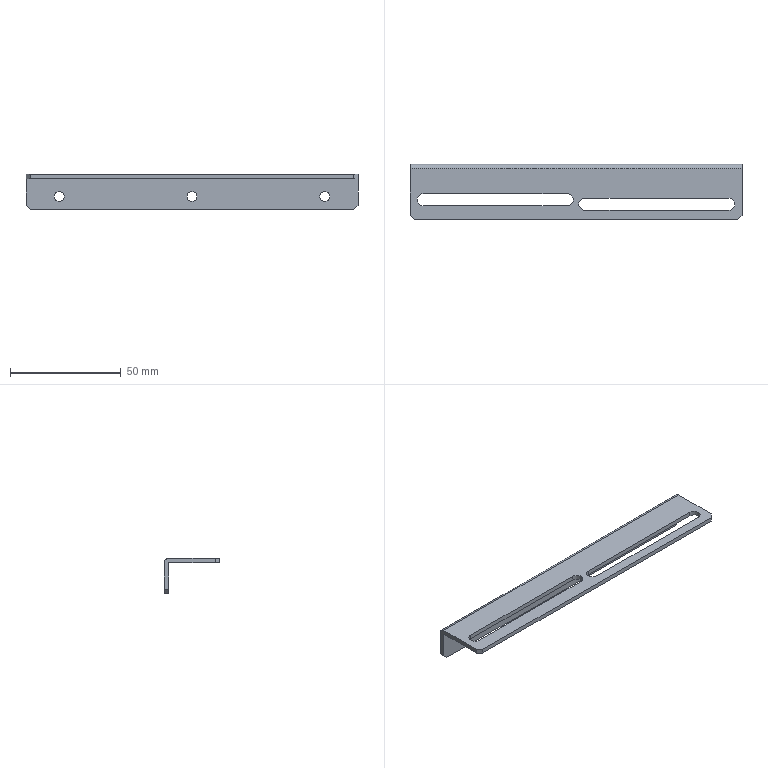Part | SolidWorks | features ICE 4, Chamfer 3, HoleWzd 3, Extrusion 1, Fillet 1 | 1 solid | 29 faces | box 150 x 25 x 16 mm | volume 9935 mm3 | plane 16 | cylinder 13 | commonest cylinder face diameters 4.5 x6 5.5 x6 4 x1
STEP:
#1=CARTESIAN_POINT('',(0.,10.5,5.75));
#2=VERTEX_POINT('',#1);
#3=CARTESIAN_POINT('',(0.,10.5,10.25));
#4=VERTEX_POINT('',#3);
#5=CARTESIAN_POINT('',(0.,10.5,8.));
#6=DIRECTION('',(0.,1.,0.));
#7=DIRECTION('',(0.,0.,1.));
#8=AXIS2_PLACEMENT_3D('',#5,#6,#7);
#9=CIRCLE('',#8,2.25);
#10=EDGE_CURVE('',#2,#4,#9,.T.);
#11=ORIENTED_EDGE('',*,*,#10,.F.);
#12=CARTESIAN_POINT('',(0.,12.5,5.75));
#13=VERTEX_POINT('',#12);
#14=CARTESIAN_POINT('',(0.,12.5,5.75));
#15=DIRECTION('',(0.,1.,0.));
#16=VECTOR('',#15,1000.);
#17=LINE('',#14,#16);
#18=EDGE_CURVE('',#2,#13,#17,.T.);
#19=ORIENTED_EDGE('',*,*,#18,.T.);
#20=CARTESIAN_POINT('',(0.,12.5,10.25));
#21=VERTEX_POINT('',#20);
#22=CARTESIAN_POINT('',(0.,12.5,8.));
#23=DIRECTION('',(0.,1.,0.));
#24=DIRECTION('',(0.,0.,1.));
#25=AXIS2_PLACEMENT_3D('',#22,#23,#24);
#26=CIRCLE('',#25,2.25);
#27=EDGE_CURVE('',#13,#21,#26,.T.);
#28=ORIENTED_EDGE('',*,*,#27,.T.);
#29=CARTESIAN_POINT('',(0.,12.5,10.25));
#30=DIRECTION('',(0.,1.,0.));
#31=VECTOR('',#30,1000.);
#32=LINE('',#29,#31);
#33=EDGE_CURVE('',#4,#21,#32,.T.);
#34=ORIENTED_EDGE('',*,*,#33,.F.);
#35=EDGE_LOOP('',(#11,#19,#28,#34));
#36=FACE_OUTER_BOUND('',#35,.T.);
#37=CARTESIAN_POINT('',(0.,12.5,8.));
#38=DIRECTION('',(0.,1.,0.));
#39=DIRECTION('',(0.,0.,1.));
#40=AXIS2_PLACEMENT_3D('',#37,#38,#39);
#41=CYLINDRICAL_SURFACE('',#40,2.25);
#42=ADVANCED_FACE('',(#36),#41,.F.);
#43=CARTESIAN_POINT('',(-60.,10.5,5.75));
#44=VERTEX_POINT('',#43);
#45=CARTESIAN_POINT('',(-60.,10.5,10.25));
#46=VERTEX_POINT('',#45);
#47=CARTESIAN_POINT('',(-60.,10.5,8.));
#48=DIRECTION('',(0.,1.,0.));
#49=DIRECTION('',(0.,0.,1.));
#50=AXIS2_PLACEMENT_3D('',#47,#48,#49);
#51=CIRCLE('',#50,2.25);
#52=EDGE_CURVE('',#44,#46,#51,.T.);
#53=ORIENTED_EDGE('',*,*,#52,.F.);
#54=CARTESIAN_POINT('',(-60.,12.5,5.75));
#55=VERTEX_POINT('',#54);
#56=CARTESIAN_POINT('',(-60.,12.5,5.75));
#57=DIRECTION('',(0.,1.,0.));
#58=VECTOR('',#57,1000.);
#59=LINE('',#56,#58);
#60=EDGE_CURVE('',#44,#55,#59,.T.);
#61=ORIENTED_EDGE('',*,*,#60,.T.);
#62=CARTESIAN_POINT('',(-60.,12.5,10.25));
#63=VERTEX_POINT('',#62);
#64=CARTESIAN_POINT('',(-60.,12.5,8.));
#65=DIRECTION('',(0.,1.,0.));
#66=DIRECTION('',(0.,0.,1.));
#67=AXIS2_PLACEMENT_3D('',#64,#65,#66);
#68=CIRCLE('',#67,2.25);
#69=EDGE_CURVE('',#55,#63,#68,.T.);
#70=ORIENTED_EDGE('',*,*,#69,.T.);
#71=CARTESIAN_POINT('',(-60.,12.5,10.25));
#72=DIRECTION('',(0.,1.,0.));
#73=VECTOR('',#72,1000.);
#74=LINE('',#71,#73);
#75=EDGE_CURVE('',#46,#63,#74,.T.);
#76=ORIENTED_EDGE('',*,*,#75,.F.);
#77=EDGE_LOOP('',(#53,#61,#70,#76));
#78=FACE_OUTER_BOUND('',#77,.T.);
#79=CARTESIAN_POINT('',(-60.,12.5,8.));
#80=DIRECTION('',(0.,1.,0.));
#81=DIRECTION('',(0.,0.,1.));
#82=AXIS2_PLACEMENT_3D('',#79,#80,#81);
#83=CYLINDRICAL_SURFACE('',#82,2.25);
#84=ADVANCED_FACE('',(#78),#83,.F.);
#85=CARTESIAN_POINT('',(60.,10.5,5.75));
#86=VERTEX_POINT('',#85);
#87=CARTESIAN_POINT('',(60.,10.5,10.25));
#88=VERTEX_POINT('',#87);
#89=CARTESIAN_POINT('',(60.,10.5,8.));
#90=DIRECTION('',(0.,1.,0.));
#91=DIRECTION('',(0.,0.,1.));
#92=AXIS2_PLACEMENT_3D('',#89,#90,#91);
#93=CIRCLE('',#92,2.25);
#94=EDGE_CURVE('',#86,#88,#93,.T.);
#95=ORIENTED_EDGE('',*,*,#94,.F.);
#96=CARTESIAN_POINT('',(60.,12.5,5.75));
#97=VERTEX_POINT('',#96);
#98=CARTESIAN_POINT('',(60.,12.5,5.75));
#99=DIRECTION('',(0.,1.,0.));
#100=VECTOR('',#99,1000.);
#101=LINE('',#98,#100);
#102=EDGE_CURVE('',#86,#97,#101,.T.);
#103=ORIENTED_EDGE('',*,*,#102,.T.);
#104=CARTESIAN_POINT('',(60.,12.5,10.25));
#105=VERTEX_POINT('',#104);
#106=CARTESIAN_POINT('',(60.,12.5,8.));
#107=DIRECTION('',(0.,1.,0.));
#108=DIRECTION('',(0.,0.,1.));
#109=AXIS2_PLACEMENT_3D('',#106,#107,#108);
#110=CIRCLE('',#109,2.25);
#111=EDGE_CURVE('',#97,#105,#110,.T.);
#112=ORIENTED_EDGE('',*,*,#111,.T.);
#113=CARTESIAN_POINT('',(60.,12.5,10.25));
#114=DIRECTION('',(0.,1.,0.));
#115=VECTOR('',#114,1000.);
#116=LINE('',#113,#115);
#117=EDGE_CURVE('',#88,#105,#116,.T.);
#118=ORIENTED_EDGE('',*,*,#117,.F.);
#119=EDGE_LOOP('',(#95,#103,#112,#118));
#120=FACE_OUTER_BOUND('',#119,.T.);
#121=CARTESIAN_POINT('',(60.,12.5,8.));
#122=DIRECTION('',(0.,1.,0.));
#123=DIRECTION('',(0.,0.,1.));
#124=AXIS2_PLACEMENT_3D('',#121,#122,#123);
#125=CYLINDRICAL_SURFACE('',#124,2.25);
#126=ADVANCED_FACE('',(#120),#125,.F.);
#127=CARTESIAN_POINT('',(-1.25,-3.5,16.));
#128=VERTEX_POINT('',#127);
#129=CARTESIAN_POINT('',(-4.,-0.75,16.));
#130=VERTEX_POINT('',#129);
#131=CARTESIAN_POINT('',(-4.,-3.5,16.));
#132=DIRECTION('',(0.,0.,1.));
#133=DIRECTION('',(1.,0.,0.));
#134=AXIS2_PLACEMENT_3D('',#131,#132,#133);
#135=CIRCLE('',#134,2.75);
#136=EDGE_CURVE('',#128,#130,#135,.T.);
#137=ORIENTED_EDGE('',*,*,#136,.F.);
#138=CARTESIAN_POINT('',(-1.25,-3.5,18.));
#139=VERTEX_POINT('',#138);
#140=CARTESIAN_POINT('',(-1.25,-3.5,0.));
#141=DIRECTION('',(0.,0.,1.));
#142=VECTOR('',#141,1000.);
#143=LINE('',#140,#142);
#144=EDGE_CURVE('',#128,#139,#143,.T.);
#145=ORIENTED_EDGE('',*,*,#144,.T.);
#146=CARTESIAN_POINT('',(-4.,-0.75,18.));
#147=VERTEX_POINT('',#146);
#148=CARTESIAN_POINT('',(-4.,-3.5,18.));
#149=DIRECTION('',(0.,0.,1.));
#150=DIRECTION('',(1.,0.,0.));
#151=AXIS2_PLACEMENT_3D('',#148,#149,#150);
#152=CIRCLE('',#151,2.75);
#153=EDGE_CURVE('',#139,#147,#152,.T.);
#154=ORIENTED_EDGE('',*,*,#153,.T.);
#155=CARTESIAN_POINT('',(-4.,-0.75,0.));
#156=DIRECTION('',(0.,0.,1.));
#157=VECTOR('',#156,1000.);
#158=LINE('',#155,#157);
#159=EDGE_CURVE('',#130,#147,#158,.T.);
#160=ORIENTED_EDGE('',*,*,#159,.F.);
#161=EDGE_LOOP('',(#137,#145,#154,#160));
#162=FACE_OUTER_BOUND('',#161,.T.);
#163=CARTESIAN_POINT('',(-4.,-3.5,0.));
#164=DIRECTION('',(0.,0.,1.));
#165=DIRECTION('',(1.,0.,0.));
#166=AXIS2_PLACEMENT_3D('',#163,#164,#165);
#167=CYLINDRICAL_SURFACE('',#166,2.75);
#168=ADVANCED_FACE('',(#162),#167,.F.);
#169=CARTESIAN_POINT('',(1.25,-5.5,18.));
#170=VERTEX_POINT('',#169);
#171=CARTESIAN_POINT('',(4.,-2.75,18.));
#172=VERTEX_POINT('',#171);
#173=CARTESIAN_POINT('',(4.,-5.5,18.));
#174=DIRECTION('',(0.,0.,-1.));
#175=DIRECTION('',(-1.,0.,0.));
#176=AXIS2_PLACEMENT_3D('',#173,#174,#175);
#177=CIRCLE('',#176,2.75);
#178=EDGE_CURVE('',#170,#172,#177,.T.);
#179=ORIENTED_EDGE('',*,*,#178,.F.);
#180=CARTESIAN_POINT('',(1.25,-5.5,16.));
#181=VERTEX_POINT('',#180);
#182=CARTESIAN_POINT('',(1.25,-5.5,18.));
#183=DIRECTION('',(0.,0.,-1.));
#184=VECTOR('',#183,1000.);
#185=LINE('',#182,#184);
#186=EDGE_CURVE('',#170,#181,#185,.T.);
#187=ORIENTED_EDGE('',*,*,#186,.T.);
#188=CARTESIAN_POINT('',(4.,-2.75,16.));
#189=VERTEX_POINT('',#188);
#190=CARTESIAN_POINT('',(4.,-5.5,16.));
#191=DIRECTION('',(0.,0.,-1.));
#192=DIRECTION('',(-1.,0.,0.));
#193=AXIS2_PLACEMENT_3D('',#190,#191,#192);
#194=CIRCLE('',#193,2.75);
#195=EDGE_CURVE('',#181,#189,#194,.T.);
#196=ORIENTED_EDGE('',*,*,#195,.T.);
#197=CARTESIAN_POINT('',(4.,-2.75,18.));
#198=DIRECTION('',(0.,0.,-1.));
#199=VECTOR('',#198,1000.);
#200=LINE('',#197,#199);
#201=EDGE_CURVE('',#172,#189,#200,.T.);
#202=ORIENTED_EDGE('',*,*,#201,.F.);
#203=EDGE_LOOP('',(#179,#187,#196,#202));
#204=FACE_OUTER_BOUND('',#203,.T.);
#205=CARTESIAN_POINT('',(4.,-5.5,18.));
#206=DIRECTION('',(0.,0.,-1.));
#207=DIRECTION('',(-1.,0.,0.));
#208=AXIS2_PLACEMENT_3D('',#205,#206,#207);
#209=CYLINDRICAL_SURFACE('',#208,2.75);
#210=ADVANCED_FACE('',(#204),#209,.F.);
#211=CARTESIAN_POINT('',(-75.,12.5,16.));
#212=VERTEX_POINT('',#211);
#213=CARTESIAN_POINT('',(-75.,12.5,4.));
#214=VERTEX_POINT('',#213);
#215=CARTESIAN_POINT('',(-75.,12.5,18.));
#216=DIRECTION('',(0.,0.,-1.));
#217=VECTOR('',#216,1000.);
#218=LINE('',#215,#217);
#219=EDGE_CURVE('',#212,#214,#218,.T.);
#220=ORIENTED_EDGE('',*,*,#219,.T.);
#221=CARTESIAN_POINT('',(-75.,10.5,4.));
#222=VERTEX_POINT('',#221);
#223=CARTESIAN_POINT('',(-75.,10.5,4.));
#224=DIRECTION('',(0.,-1.,0.));
#225=VECTOR('',#224,1000.);
#226=LINE('',#223,#225);
#227=EDGE_CURVE('',#214,#222,#226,.T.);
#228=ORIENTED_EDGE('',*,*,#227,.T.);
#229=CARTESIAN_POINT('',(-75.,10.5,16.));
#230=VERTEX_POINT('',#229);
#231=CARTESIAN_POINT('',(-75.,10.5,16.));
#232=DIRECTION('',(0.,0.,-1.));
#233=VECTOR('',#232,1000.);
#234=LINE('',#231,#233);
#235=EDGE_CURVE('',#230,#222,#234,.T.);
#236=ORIENTED_EDGE('',*,*,#235,.F.);
#237=CARTESIAN_POINT('',(-75.,-10.5,16.));
#238=VERTEX_POINT('',#237);
#239=CARTESIAN_POINT('',(-75.,-12.5,16.));
#240=DIRECTION('',(0.,1.,0.));
#241=VECTOR('',#240,1000.);
#242=LINE('',#239,#241);
#243=EDGE_CURVE('',#238,#230,#242,.T.);
#244=ORIENTED_EDGE('',*,*,#243,.F.);
#245=CARTESIAN_POINT('',(-75.,-10.5,18.));
#246=VERTEX_POINT('',#245);
#247=CARTESIAN_POINT('',(-75.,-10.5,18.));
#248=DIRECTION('',(0.,0.,1.));
#249=VECTOR('',#248,1000.);
#250=LINE('',#247,#249);
#251=EDGE_CURVE('',#238,#246,#250,.T.);
#252=ORIENTED_EDGE('',*,*,#251,.T.);
#253=CARTESIAN_POINT('',(-75.,10.5,18.));
#254=VERTEX_POINT('',#253);
#255=CARTESIAN_POINT('',(-75.,-12.5,18.));
#256=DIRECTION('',(0.,1.,0.));
#257=VECTOR('',#256,1000.);
#258=LINE('',#255,#257);
#259=EDGE_CURVE('',#246,#254,#258,.T.);
#260=ORIENTED_EDGE('',*,*,#259,.T.);
#261=CARTESIAN_POINT('',(-75.,10.5,16.));
#262=DIRECTION('',(-1.,0.,0.));
#263=DIRECTION('',(0.,0.,1.));
#264=AXIS2_PLACEMENT_3D('',#261,#262,#263);
#265=CIRCLE('',#264,2.);
#266=EDGE_CURVE('',#254,#212,#265,.T.);
#267=ORIENTED_EDGE('',*,*,#266,.T.);
#268=EDGE_LOOP('',(#220,#228,#236,#244,#252,#260,#267));
#269=FACE_OUTER_BOUND('',#268,.T.);
#270=CARTESIAN_POINT('',(-75.,-12.5,18.));
#271=DIRECTION('',(-1.,0.,0.));
#272=DIRECTION('',(0.,0.,1.));
#273=AXIS2_PLACEMENT_3D('',#270,#271,#272);
#274=PLANE('',#273);
#275=ADVANCED_FACE('',(#269),#274,.T.);
#276=CARTESIAN_POINT('',(73.,-12.5,18.));
#277=VERTEX_POINT('',#276);
#278=CARTESIAN_POINT('',(-73.,-12.5,18.));
#279=VERTEX_POINT('',#278);
#280=CARTESIAN_POINT('',(75.,-12.5,18.));
#281=DIRECTION('',(-1.,0.,0.));
#282=VECTOR('',#281,1000.);
#283=LINE('',#280,#282);
#284=EDGE_CURVE('',#277,#279,#283,.T.);
#285=ORIENTED_EDGE('',*,*,#284,.T.);
#286=CARTESIAN_POINT('',(-73.,-12.5,16.));
#287=VERTEX_POINT('',#286);
#288=CARTESIAN_POINT('',(-73.,-12.5,18.));
#289=DIRECTION('',(0.,0.,-1.));
#290=VECTOR('',#289,1000.);
#291=LINE('',#288,#290);
#292=EDGE_CURVE('',#279,#287,#291,.T.);
#293=ORIENTED_EDGE('',*,*,#292,.T.);
#294=CARTESIAN_POINT('',(73.,-12.5,16.));
#295=VERTEX_POINT('',#294);
#296=CARTESIAN_POINT('',(75.,-12.5,16.));
#297=DIRECTION('',(-1.,0.,0.));
#298=VECTOR('',#297,1000.);
#299=LINE('',#296,#298);
#300=EDGE_CURVE('',#295,#287,#299,.T.);
#301=ORIENTED_EDGE('',*,*,#300,.F.);
#302=CARTESIAN_POINT('',(73.,-12.5,18.));
#303=DIRECTION('',(0.,0.,1.));
#304=VECTOR('',#303,1000.);
#305=LINE('',#302,#304);
#306=EDGE_CURVE('',#295,#277,#305,.T.);
#307=ORIENTED_EDGE('',*,*,#306,.T.);
#308=EDGE_LOOP('',(#285,#293,#301,#307));
#309=FACE_OUTER_BOUND('',#308,.T.);
#310=CARTESIAN_POINT('',(75.,-12.5,18.));
#311=DIRECTION('',(0.,-1.,0.));
#312=DIRECTION('',(0.,0.,-1.));
#313=AXIS2_PLACEMENT_3D('',#310,#311,#312);
#314=PLANE('',#313);
#315=ADVANCED_FACE('',(#309),#314,.T.);
#316=CARTESIAN_POINT('',(75.,10.5,16.));
#317=VERTEX_POINT('',#316);
#318=CARTESIAN_POINT('',(75.,10.5,4.));
#319=VERTEX_POINT('',#318);
#320=CARTESIAN_POINT('',(75.,10.5,16.));
#321=DIRECTION('',(0.,0.,-1.));
#322=VECTOR('',#321,1000.);
#323=LINE('',#320,#322);
#324=EDGE_CURVE('',#317,#319,#323,.T.);
#325=ORIENTED_EDGE('',*,*,#324,.T.);
#326=CARTESIAN_POINT('',(75.,12.5,4.));
#327=VERTEX_POINT('',#326);
#328=CARTESIAN_POINT('',(75.,12.5,4.));
#329=DIRECTION('',(0.,1.,0.));
#330=VECTOR('',#329,1000.);
#331=LINE('',#328,#330);
#332=EDGE_CURVE('',#319,#327,#331,.T.);
#333=ORIENTED_EDGE('',*,*,#332,.T.);
#334=CARTESIAN_POINT('',(75.,12.5,16.));
#335=VERTEX_POINT('',#334);
#336=CARTESIAN_POINT('',(75.,12.5,18.));
#337=DIRECTION('',(0.,0.,-1.));
#338=VECTOR('',#337,1000.);
#339=LINE('',#336,#338);
#340=EDGE_CURVE('',#335,#327,#339,.T.);
#341=ORIENTED_EDGE('',*,*,#340,.F.);
#342=CARTESIAN_POINT('',(75.,10.5,18.));
#343=VERTEX_POINT('',#342);
#344=CARTESIAN_POINT('',(75.,10.5,16.));
#345=DIRECTION('',(1.,0.,0.));
#346=DIRECTION('',(0.,0.,-1.));
#347=AXIS2_PLACEMENT_3D('',#344,#345,#346);
#348=CIRCLE('',#347,2.);
#349=EDGE_CURVE('',#335,#343,#348,.T.);
#350=ORIENTED_EDGE('',*,*,#349,.T.);
#351=CARTESIAN_POINT('',(75.,-10.5,18.));
#352=VERTEX_POINT('',#351);
#353=CARTESIAN_POINT('',(75.,12.5,18.));
#354=DIRECTION('',(0.,-1.,0.));
#355=VECTOR('',#354,1000.);
#356=LINE('',#353,#355);
#357=EDGE_CURVE('',#343,#352,#356,.T.);
#358=ORIENTED_EDGE('',*,*,#357,.T.);
#359=CARTESIAN_POINT('',(75.,-10.5,16.));
#360=VERTEX_POINT('',#359);
#361=CARTESIAN_POINT('',(75.,-10.5,18.));
#362=DIRECTION('',(0.,0.,-1.));
#363=VECTOR('',#362,1000.);
#364=LINE('',#361,#363);
#365=EDGE_CURVE('',#352,#360,#364,.T.);
#366=ORIENTED_EDGE('',*,*,#365,.T.);
#367=CARTESIAN_POINT('',(75.,-12.5,16.));
#368=DIRECTION('',(0.,1.,0.));
#369=VECTOR('',#368,1000.);
#370=LINE('',#367,#369);
#371=EDGE_CURVE('',#360,#317,#370,.T.);
#372=ORIENTED_EDGE('',*,*,#371,.T.);
#373=EDGE_LOOP('',(#325,#333,#341,#350,#358,#366,#372));
#374=FACE_OUTER_BOUND('',#373,.T.);
#375=CARTESIAN_POINT('',(75.,12.5,18.));
#376=DIRECTION('',(1.,0.,0.));
#377=DIRECTION('',(0.,0.,-1.));
#378=AXIS2_PLACEMENT_3D('',#375,#376,#377);
#379=PLANE('',#378);
#380=ADVANCED_FACE('',(#374),#379,.T.);
#381=ORIENTED_EDGE('',*,*,#340,.T.);
#382=CARTESIAN_POINT('',(73.,12.5,2.));
#383=VERTEX_POINT('',#382);
#384=CARTESIAN_POINT('',(7.,12.5,-64.));
#385=DIRECTION('',(-0.7071,0.,-0.7071));
#386=VECTOR('',#385,1000.);
#387=LINE('',#384,#386);
#388=EDGE_CURVE('',#327,#383,#387,.T.);
#389=ORIENTED_EDGE('',*,*,#388,.T.);
#390=CARTESIAN_POINT('',(-73.,12.5,2.));
#391=VERTEX_POINT('',#390);
#392=CARTESIAN_POINT('',(75.,12.5,2.));
#393=DIRECTION('',(1.,0.,0.));
#394=VECTOR('',#393,1000.);
#395=LINE('',#392,#394);
#396=EDGE_CURVE('',#391,#383,#395,.T.);
#397=ORIENTED_EDGE('',*,*,#396,.F.);
#398=CARTESIAN_POINT('',(-82.,12.5,11.));
#399=DIRECTION('',(-0.7071,0.,0.7071));
#400=VECTOR('',#399,1000.);
#401=LINE('',#398,#400);
#402=EDGE_CURVE('',#391,#214,#401,.T.);
#403=ORIENTED_EDGE('',*,*,#402,.T.);
#404=ORIENTED_EDGE('',*,*,#219,.F.);
#405=CARTESIAN_POINT('',(75.,12.5,16.));
#406=DIRECTION('',(1.,0.,0.));
#407=VECTOR('',#406,1000.);
#408=LINE('',#405,#407);
#409=EDGE_CURVE('',#212,#335,#408,.T.);
#410=ORIENTED_EDGE('',*,*,#409,.T.);
#411=EDGE_LOOP('',(#381,#389,#397,#403,#404,#410));
#412=FACE_OUTER_BOUND('',#411,.T.);
#413=CARTESIAN_POINT('',(0.,12.5,8.));
#414=DIRECTION('',(0.,1.,0.));
#415=DIRECTION('',(0.,0.,1.));
#416=AXIS2_PLACEMENT_3D('',#413,#414,#415);
#417=CIRCLE('',#416,2.25);
#418=EDGE_CURVE('',#21,#13,#417,.T.);
#419=ORIENTED_EDGE('',*,*,#418,.F.);
#420=ORIENTED_EDGE('',*,*,#27,.F.);
#421=EDGE_LOOP('',(#419,#420));
#422=FACE_BOUND('',#421,.T.);
#423=CARTESIAN_POINT('',(-60.,12.5,8.));
#424=DIRECTION('',(0.,1.,0.));
#425=DIRECTION('',(0.,0.,1.));
#426=AXIS2_PLACEMENT_3D('',#423,#424,#425);
#427=CIRCLE('',#426,2.25);
#428=EDGE_CURVE('',#63,#55,#427,.T.);
#429=ORIENTED_EDGE('',*,*,#428,.F.);
#430=ORIENTED_EDGE('',*,*,#69,.F.);
#431=EDGE_LOOP('',(#429,#430));
#432=FACE_BOUND('',#431,.T.);
#433=CARTESIAN_POINT('',(60.,12.5,8.));
#434=DIRECTION('',(0.,1.,0.));
#435=DIRECTION('',(0.,0.,1.));
#436=AXIS2_PLACEMENT_3D('',#433,#434,#435);
#437=CIRCLE('',#436,2.25);
#438=EDGE_CURVE('',#105,#97,#437,.T.);
#439=ORIENTED_EDGE('',*,*,#438,.F.);
#440=ORIENTED_EDGE('',*,*,#111,.F.);
#441=EDGE_LOOP('',(#439,#440));
#442=FACE_BOUND('',#441,.T.);
#443=CARTESIAN_POINT('',(-75.,12.5,18.));
#444=DIRECTION('',(0.,1.,0.));
#445=DIRECTION('',(0.,0.,1.));
#446=AXIS2_PLACEMENT_3D('',#443,#444,#445);
#447=PLANE('',#446);
#448=ADVANCED_FACE('',(#412,#422,#432,#442),#447,.T.);
#449=CARTESIAN_POINT('',(-69.,-6.25,18.));
#450=VERTEX_POINT('',#449);
#451=CARTESIAN_POINT('',(-4.,-6.25,18.));
#452=VERTEX_POINT('',#451);
#453=CARTESIAN_POINT('',(-69.,-6.25,18.));
#454=DIRECTION('',(1.,0.,0.));
#455=VECTOR('',#454,1000.);
#456=LINE('',#453,#455);
#457=EDGE_CURVE('',#450,#452,#456,.T.);
#458=ORIENTED_EDGE('',*,*,#457,.F.);
#459=CARTESIAN_POINT('',(-69.,-0.75,18.));
#460=VERTEX_POINT('',#459);
#461=CARTESIAN_POINT('',(-69.,-3.5,18.));
#462=DIRECTION('',(0.,0.,1.));
#463=DIRECTION('',(1.,0.,0.));
#464=AXIS2_PLACEMENT_3D('',#461,#462,#463);
#465=CIRCLE('',#464,2.75);
#466=EDGE_CURVE('',#460,#450,#465,.T.);
#467=ORIENTED_EDGE('',*,*,#466,.F.);
#468=CARTESIAN_POINT('',(-4.,-0.75,18.));
#469=DIRECTION('',(-1.,0.,0.));
#470=VECTOR('',#469,1000.);
#471=LINE('',#468,#470);
#472=EDGE_CURVE('',#147,#460,#471,.T.);
#473=ORIENTED_EDGE('',*,*,#472,.F.);
#474=ORIENTED_EDGE('',*,*,#153,.F.);
#475=CARTESIAN_POINT('',(-4.,-3.5,18.));
#476=DIRECTION('',(0.,0.,1.));
#477=DIRECTION('',(1.,0.,0.));
#478=AXIS2_PLACEMENT_3D('',#475,#476,#477);
#479=CIRCLE('',#478,2.75);
#480=EDGE_CURVE('',#452,#139,#479,.T.);
#481=ORIENTED_EDGE('',*,*,#480,.F.);
#482=EDGE_LOOP('',(#458,#467,#473,#474,#481));
#483=FACE_BOUND('',#482,.T.);
#484=CARTESIAN_POINT('',(69.,-8.25,18.));
#485=VERTEX_POINT('',#484);
#486=CARTESIAN_POINT('',(4.,-8.25,18.));
#487=VERTEX_POINT('',#486);
#488=CARTESIAN_POINT('',(69.,-8.25,18.));
#489=DIRECTION('',(-1.,0.,0.));
#490=VECTOR('',#489,1000.);
#491=LINE('',#488,#490);
#492=EDGE_CURVE('',#485,#487,#491,.T.);
#493=ORIENTED_EDGE('',*,*,#492,.T.);
#494=CARTESIAN_POINT('',(4.,-5.5,18.));
#495=DIRECTION('',(0.,0.,-1.));
#496=DIRECTION('',(-1.,0.,0.));
#497=AXIS2_PLACEMENT_3D('',#494,#495,#496);
#498=CIRCLE('',#497,2.75);
#499=EDGE_CURVE('',#487,#170,#498,.T.);
#500=ORIENTED_EDGE('',*,*,#499,.T.);
#501=ORIENTED_EDGE('',*,*,#178,.T.);
#502=CARTESIAN_POINT('',(69.,-2.75,18.));
#503=VERTEX_POINT('',#502);
#504=CARTESIAN_POINT('',(4.,-2.75,18.));
#505=DIRECTION('',(1.,0.,0.));
#506=VECTOR('',#505,1000.);
#507=LINE('',#504,#506);
#508=EDGE_CURVE('',#172,#503,#507,.T.);
#509=ORIENTED_EDGE('',*,*,#508,.T.);
#510=CARTESIAN_POINT('',(69.,-5.5,18.));
#511=DIRECTION('',(0.,0.,-1.));
#512=DIRECTION('',(-1.,0.,0.));
#513=AXIS2_PLACEMENT_3D('',#510,#511,#512);
#514=CIRCLE('',#513,2.75);
#515=EDGE_CURVE('',#503,#485,#514,.T.);
#516=ORIENTED_EDGE('',*,*,#515,.T.);
#517=EDGE_LOOP('',(#493,#500,#501,#509,#516));
#518=FACE_BOUND('',#517,.T.);
#519=ORIENTED_EDGE('',*,*,#357,.F.);
#520=CARTESIAN_POINT('',(-75.,10.5,18.));
#521=DIRECTION('',(-1.,0.,0.));
#522=VECTOR('',#521,1000.);
#523=LINE('',#520,#522);
#524=EDGE_CURVE('',#343,#254,#523,.T.);
#525=ORIENTED_EDGE('',*,*,#524,.T.);
#526=ORIENTED_EDGE('',*,*,#259,.F.);
#527=CARTESIAN_POINT('',(-73.,-12.5,18.));
#528=DIRECTION('',(0.7071,-0.7071,0.));
#529=VECTOR('',#528,1000.);
#530=LINE('',#527,#529);
#531=EDGE_CURVE('',#246,#279,#530,.T.);
#532=ORIENTED_EDGE('',*,*,#531,.T.);
#533=ORIENTED_EDGE('',*,*,#284,.F.);
#534=CARTESIAN_POINT('',(75.,-10.5,18.));
#535=DIRECTION('',(0.7071,0.7071,0.));
#536=VECTOR('',#535,1000.);
#537=LINE('',#534,#536);
#538=EDGE_CURVE('',#277,#352,#537,.T.);
#539=ORIENTED_EDGE('',*,*,#538,.T.);
#540=EDGE_LOOP('',(#519,#525,#526,#532,#533,#539));
#541=FACE_OUTER_BOUND('',#540,.T.);
#542=CARTESIAN_POINT('',(-75.,12.5,18.));
#543=DIRECTION('',(0.,0.,-1.));
#544=DIRECTION('',(-1.,0.,0.));
#545=AXIS2_PLACEMENT_3D('',#542,#543,#544);
#546=PLANE('',#545);
#547=ADVANCED_FACE('',(#483,#518,#541),#546,.F.);
#548=CARTESIAN_POINT('',(0.,10.5,8.));
#549=DIRECTION('',(0.,1.,0.));
#550=DIRECTION('',(0.,0.,1.));
#551=AXIS2_PLACEMENT_3D('',#548,#549,#550);
#552=CIRCLE('',#551,2.25);
#553=EDGE_CURVE('',#4,#2,#552,.T.);
#554=ORIENTED_EDGE('',*,*,#553,.T.);
#555=ORIENTED_EDGE('',*,*,#10,.T.);
#556=EDGE_LOOP('',(#554,#555));
#557=FACE_BOUND('',#556,.T.);
#558=CARTESIAN_POINT('',(-60.,10.5,8.));
#559=DIRECTION('',(0.,1.,0.));
#560=DIRECTION('',(0.,0.,1.));
#561=AXIS2_PLACEMENT_3D('',#558,#559,#560);
#562=CIRCLE('',#561,2.25);
#563=EDGE_CURVE('',#46,#44,#562,.T.);
#564=ORIENTED_EDGE('',*,*,#563,.T.);
#565=ORIENTED_EDGE('',*,*,#52,.T.);
#566=EDGE_LOOP('',(#564,#565));
#567=FACE_BOUND('',#566,.T.);
#568=CARTESIAN_POINT('',(60.,10.5,8.));
#569=DIRECTION('',(0.,1.,0.));
#570=DIRECTION('',(0.,0.,1.));
#571=AXIS2_PLACEMENT_3D('',#568,#569,#570);
#572=CIRCLE('',#571,2.25);
#573=EDGE_CURVE('',#88,#86,#572,.T.);
#574=ORIENTED_EDGE('',*,*,#573,.T.);
#575=ORIENTED_EDGE('',*,*,#94,.T.);
#576=EDGE_LOOP('',(#574,#575));
#577=FACE_BOUND('',#576,.T.);
#578=CARTESIAN_POINT('',(-73.,10.5,2.));
#579=VERTEX_POINT('',#578);
#580=CARTESIAN_POINT('',(73.,10.5,2.));
#581=VERTEX_POINT('',#580);
#582=CARTESIAN_POINT('',(75.,10.5,2.));
#583=DIRECTION('',(1.,0.,0.));
#584=VECTOR('',#583,1000.);
#585=LINE('',#582,#584);
#586=EDGE_CURVE('',#579,#581,#585,.T.);
#587=ORIENTED_EDGE('',*,*,#586,.T.);
#588=CARTESIAN_POINT('',(75.,10.5,4.));
#589=DIRECTION('',(0.7071,0.,0.7071));
#590=VECTOR('',#589,1000.);
#591=LINE('',#588,#590);
#592=EDGE_CURVE('',#581,#319,#591,.T.);
#593=ORIENTED_EDGE('',*,*,#592,.T.);
#594=ORIENTED_EDGE('',*,*,#324,.F.);
#595=CARTESIAN_POINT('',(75.,10.5,16.));
#596=DIRECTION('',(-1.,0.,0.));
#597=VECTOR('',#596,1000.);
#598=LINE('',#595,#597);
#599=EDGE_CURVE('',#317,#230,#598,.T.);
#600=ORIENTED_EDGE('',*,*,#599,.T.);
#601=ORIENTED_EDGE('',*,*,#235,.T.);
#602=CARTESIAN_POINT('',(-73.,10.5,2.));
#603=DIRECTION('',(0.7071,0.,-0.7071));
#604=VECTOR('',#603,1000.);
#605=LINE('',#602,#604);
#606=EDGE_CURVE('',#222,#579,#605,.T.);
#607=ORIENTED_EDGE('',*,*,#606,.T.);
#608=EDGE_LOOP('',(#587,#593,#594,#600,#601,#607));
#609=FACE_OUTER_BOUND('',#608,.T.);
#610=CARTESIAN_POINT('',(75.,10.5,16.));
#611=DIRECTION('',(0.,1.,0.));
#612=DIRECTION('',(0.,0.,1.));
#613=AXIS2_PLACEMENT_3D('',#610,#611,#612);
#614=PLANE('',#613);
#615=ADVANCED_FACE('',(#557,#567,#577,#609),#614,.F.);
#616=CARTESIAN_POINT('',(-69.,-0.75,16.));
#617=VERTEX_POINT('',#616);
#618=CARTESIAN_POINT('',(75.,-0.75,16.));
#619=DIRECTION('',(-1.,0.,0.));
#620=VECTOR('',#619,1000.);
#621=LINE('',#618,#620);
#622=EDGE_CURVE('',#130,#617,#621,.T.);
#623=ORIENTED_EDGE('',*,*,#622,.T.);
#624=CARTESIAN_POINT('',(-69.,-6.25,16.));
#625=VERTEX_POINT('',#624);
#626=CARTESIAN_POINT('',(-69.,-3.5,16.));
#627=DIRECTION('',(0.,0.,1.));
#628=DIRECTION('',(1.,0.,0.));
#629=AXIS2_PLACEMENT_3D('',#626,#627,#628);
#630=CIRCLE('',#629,2.75);
#631=EDGE_CURVE('',#617,#625,#630,.T.);
#632=ORIENTED_EDGE('',*,*,#631,.T.);
#633=CARTESIAN_POINT('',(-4.,-6.25,16.));
#634=VERTEX_POINT('',#633);
#635=CARTESIAN_POINT('',(75.,-6.25,16.));
#636=DIRECTION('',(1.,0.,0.));
#637=VECTOR('',#636,1000.);
#638=LINE('',#635,#637);
#639=EDGE_CURVE('',#625,#634,#638,.T.);
#640=ORIENTED_EDGE('',*,*,#639,.T.);
#641=CARTESIAN_POINT('',(-4.,-3.5,16.));
#642=DIRECTION('',(0.,0.,1.));
#643=DIRECTION('',(1.,0.,0.));
#644=AXIS2_PLACEMENT_3D('',#641,#642,#643);
#645=CIRCLE('',#644,2.75);
#646=EDGE_CURVE('',#634,#128,#645,.T.);
#647=ORIENTED_EDGE('',*,*,#646,.T.);
#648=ORIENTED_EDGE('',*,*,#136,.T.);
#649=EDGE_LOOP('',(#623,#632,#640,#647,#648));
#650=FACE_BOUND('',#649,.T.);
#651=CARTESIAN_POINT('',(69.,-2.75,16.));
#652=VERTEX_POINT('',#651);
#653=CARTESIAN_POINT('',(4.,-2.75,16.));
#654=DIRECTION('',(1.,0.,0.));
#655=VECTOR('',#654,1000.);
#656=LINE('',#653,#655);
#657=EDGE_CURVE('',#189,#652,#656,.T.);
#658=ORIENTED_EDGE('',*,*,#657,.F.);
#659=ORIENTED_EDGE('',*,*,#195,.F.);
#660=CARTESIAN_POINT('',(4.,-8.25,16.));
#661=VERTEX_POINT('',#660);
#662=CARTESIAN_POINT('',(4.,-5.5,16.));
#663=DIRECTION('',(0.,0.,-1.));
#664=DIRECTION('',(-1.,0.,0.));
#665=AXIS2_PLACEMENT_3D('',#662,#663,#664);
#666=CIRCLE('',#665,2.75);
#667=EDGE_CURVE('',#661,#181,#666,.T.);
#668=ORIENTED_EDGE('',*,*,#667,.F.);
#669=CARTESIAN_POINT('',(69.,-8.25,16.));
#670=VERTEX_POINT('',#669);
#671=CARTESIAN_POINT('',(69.,-8.25,16.));
#672=DIRECTION('',(-1.,0.,0.));
#673=VECTOR('',#672,1000.);
#674=LINE('',#671,#673);
#675=EDGE_CURVE('',#670,#661,#674,.T.);
#676=ORIENTED_EDGE('',*,*,#675,.F.);
#677=CARTESIAN_POINT('',(69.,-5.5,16.));
#678=DIRECTION('',(0.,0.,-1.));
#679=DIRECTION('',(-1.,0.,0.));
#680=AXIS2_PLACEMENT_3D('',#677,#678,#679);
#681=CIRCLE('',#680,2.75);
#682=EDGE_CURVE('',#652,#670,#681,.T.);
#683=ORIENTED_EDGE('',*,*,#682,.F.);
#684=EDGE_LOOP('',(#658,#659,#668,#676,#683));
#685=FACE_BOUND('',#684,.T.);
#686=ORIENTED_EDGE('',*,*,#300,.T.);
#687=CARTESIAN_POINT('',(-73.,-12.5,16.));
#688=DIRECTION('',(-0.7071,0.7071,0.));
#689=VECTOR('',#688,1000.);
#690=LINE('',#687,#689);
#691=EDGE_CURVE('',#287,#238,#690,.T.);
#692=ORIENTED_EDGE('',*,*,#691,.T.);
#693=ORIENTED_EDGE('',*,*,#243,.T.);
#694=ORIENTED_EDGE('',*,*,#599,.F.);
#695=ORIENTED_EDGE('',*,*,#371,.F.);
#696=CARTESIAN_POINT('',(75.,-10.5,16.));
#697=DIRECTION('',(-0.7071,-0.7071,0.));
#698=VECTOR('',#697,1000.);
#699=LINE('',#696,#698);
#700=EDGE_CURVE('',#360,#295,#699,.T.);
#701=ORIENTED_EDGE('',*,*,#700,.T.);
#702=EDGE_LOOP('',(#686,#692,#693,#694,#695,#701));
#703=FACE_OUTER_BOUND('',#702,.T.);
#704=CARTESIAN_POINT('',(75.,-12.5,16.));
#705=DIRECTION('',(0.,0.,1.));
#706=DIRECTION('',(1.,0.,0.));
#707=AXIS2_PLACEMENT_3D('',#704,#705,#706);
#708=PLANE('',#707);
#709=ADVANCED_FACE('',(#650,#685,#703),#708,.F.);
#710=ORIENTED_EDGE('',*,*,#186,.F.);
#711=ORIENTED_EDGE('',*,*,#499,.F.);
#712=CARTESIAN_POINT('',(4.,-8.25,18.));
#713=DIRECTION('',(0.,0.,-1.));
#714=VECTOR('',#713,1000.);
#715=LINE('',#712,#714);
#716=EDGE_CURVE('',#487,#661,#715,.T.);
#717=ORIENTED_EDGE('',*,*,#716,.T.);
#718=ORIENTED_EDGE('',*,*,#667,.T.);
#719=EDGE_LOOP('',(#710,#711,#717,#718));
#720=FACE_OUTER_BOUND('',#719,.T.);
#721=CARTESIAN_POINT('',(4.,-5.5,18.));
#722=DIRECTION('',(0.,0.,-1.));
#723=DIRECTION('',(-1.,0.,0.));
#724=AXIS2_PLACEMENT_3D('',#721,#722,#723);
#725=CYLINDRICAL_SURFACE('',#724,2.75);
#726=ADVANCED_FACE('',(#720),#725,.F.);
#727=ORIENTED_EDGE('',*,*,#675,.T.);
#728=ORIENTED_EDGE('',*,*,#716,.F.);
#729=ORIENTED_EDGE('',*,*,#492,.F.);
#730=CARTESIAN_POINT('',(69.,-8.25,18.));
#731=DIRECTION('',(0.,0.,-1.));
#732=VECTOR('',#731,1000.);
#733=LINE('',#730,#732);
#734=EDGE_CURVE('',#485,#670,#733,.T.);
#735=ORIENTED_EDGE('',*,*,#734,.T.);
#736=EDGE_LOOP('',(#727,#728,#729,#735));
#737=FACE_OUTER_BOUND('',#736,.T.);
#738=CARTESIAN_POINT('',(69.,-8.25,18.));
#739=DIRECTION('',(0.,-1.,0.));
#740=DIRECTION('',(0.,0.,-1.));
#741=AXIS2_PLACEMENT_3D('',#738,#739,#740);
#742=PLANE('',#741);
#743=ADVANCED_FACE('',(#737),#742,.F.);
#744=ORIENTED_EDGE('',*,*,#682,.T.);
#745=ORIENTED_EDGE('',*,*,#734,.F.);
#746=ORIENTED_EDGE('',*,*,#515,.F.);
#747=CARTESIAN_POINT('',(69.,-2.75,18.));
#748=DIRECTION('',(0.,0.,-1.));
#749=VECTOR('',#748,1000.);
#750=LINE('',#747,#749);
#751=EDGE_CURVE('',#503,#652,#750,.T.);
#752=ORIENTED_EDGE('',*,*,#751,.T.);
#753=EDGE_LOOP('',(#744,#745,#746,#752));
#754=FACE_OUTER_BOUND('',#753,.T.);
#755=CARTESIAN_POINT('',(69.,-5.5,18.));
#756=DIRECTION('',(0.,0.,-1.));
#757=DIRECTION('',(-1.,0.,0.));
#758=AXIS2_PLACEMENT_3D('',#755,#756,#757);
#759=CYLINDRICAL_SURFACE('',#758,2.75);
#760=ADVANCED_FACE('',(#754),#759,.F.);
#761=ORIENTED_EDGE('',*,*,#657,.T.);
#762=ORIENTED_EDGE('',*,*,#751,.F.);
#763=ORIENTED_EDGE('',*,*,#508,.F.);
#764=ORIENTED_EDGE('',*,*,#201,.T.);
#765=EDGE_LOOP('',(#761,#762,#763,#764));
#766=FACE_OUTER_BOUND('',#765,.T.);
#767=CARTESIAN_POINT('',(4.,-2.75,18.));
#768=DIRECTION('',(0.,1.,0.));
#769=DIRECTION('',(-1.,0.,0.));
#770=AXIS2_PLACEMENT_3D('',#767,#768,#769);
#771=PLANE('',#770);
#772=ADVANCED_FACE('',(#766),#771,.F.);
#773=CARTESIAN_POINT('',(-69.,-0.75,0.));
#774=DIRECTION('',(0.,0.,1.));
#775=VECTOR('',#774,1000.);
#776=LINE('',#773,#775);
#777=EDGE_CURVE('',#617,#460,#776,.T.);
#778=ORIENTED_EDGE('',*,*,#777,.T.);
#779=ORIENTED_EDGE('',*,*,#466,.T.);
#780=CARTESIAN_POINT('',(-69.,-6.25,0.));
#781=DIRECTION('',(0.,0.,1.));
#782=VECTOR('',#781,1000.);
#783=LINE('',#780,#782);
#784=EDGE_CURVE('',#625,#450,#783,.T.);
#785=ORIENTED_EDGE('',*,*,#784,.F.);
#786=ORIENTED_EDGE('',*,*,#631,.F.);
#787=EDGE_LOOP('',(#778,#779,#785,#786));
#788=FACE_OUTER_BOUND('',#787,.T.);
#789=CARTESIAN_POINT('',(-69.,-3.5,0.));
#790=DIRECTION('',(0.,0.,1.));
#791=DIRECTION('',(1.,0.,0.));
#792=AXIS2_PLACEMENT_3D('',#789,#790,#791);
#793=CYLINDRICAL_SURFACE('',#792,2.75);
#794=ADVANCED_FACE('',(#788),#793,.F.);
#795=ORIENTED_EDGE('',*,*,#159,.T.);
#796=ORIENTED_EDGE('',*,*,#472,.T.);
#797=ORIENTED_EDGE('',*,*,#777,.F.);
#798=ORIENTED_EDGE('',*,*,#622,.F.);
#799=EDGE_LOOP('',(#795,#796,#797,#798));
#800=FACE_OUTER_BOUND('',#799,.T.);
#801=CARTESIAN_POINT('',(-4.,-0.75,0.));
#802=DIRECTION('',(0.,1.,0.));
#803=DIRECTION('',(-1.,0.,0.));
#804=AXIS2_PLACEMENT_3D('',#801,#802,#803);
#805=PLANE('',#804);
#806=ADVANCED_FACE('',(#800),#805,.F.);
#807=ORIENTED_EDGE('',*,*,#144,.F.);
#808=ORIENTED_EDGE('',*,*,#646,.F.);
#809=CARTESIAN_POINT('',(-4.,-6.25,0.));
#810=DIRECTION('',(0.,0.,1.));
#811=VECTOR('',#810,1000.);
#812=LINE('',#809,#811);
#813=EDGE_CURVE('',#634,#452,#812,.T.);
#814=ORIENTED_EDGE('',*,*,#813,.T.);
#815=ORIENTED_EDGE('',*,*,#480,.T.);
#816=EDGE_LOOP('',(#807,#808,#814,#815));
#817=FACE_OUTER_BOUND('',#816,.T.);
#818=CARTESIAN_POINT('',(-4.,-3.5,0.));
#819=DIRECTION('',(0.,0.,1.));
#820=DIRECTION('',(1.,0.,0.));
#821=AXIS2_PLACEMENT_3D('',#818,#819,#820);
#822=CYLINDRICAL_SURFACE('',#821,2.75);
#823=ADVANCED_FACE('',(#817),#822,.F.);
#824=ORIENTED_EDGE('',*,*,#784,.T.);
#825=ORIENTED_EDGE('',*,*,#457,.T.);
#826=ORIENTED_EDGE('',*,*,#813,.F.);
#827=ORIENTED_EDGE('',*,*,#639,.F.);
#828=EDGE_LOOP('',(#824,#825,#826,#827));
#829=FACE_OUTER_BOUND('',#828,.T.);
#830=CARTESIAN_POINT('',(-69.,-6.25,0.));
#831=DIRECTION('',(0.,-1.,0.));
#832=DIRECTION('',(0.,0.,-1.));
#833=AXIS2_PLACEMENT_3D('',#830,#831,#832);
#834=PLANE('',#833);
#835=ADVANCED_FACE('',(#829),#834,.F.);
#836=ORIENTED_EDGE('',*,*,#102,.F.);
#837=ORIENTED_EDGE('',*,*,#573,.F.);
#838=ORIENTED_EDGE('',*,*,#117,.T.);
#839=ORIENTED_EDGE('',*,*,#438,.T.);
#840=EDGE_LOOP('',(#836,#837,#838,#839));
#841=FACE_OUTER_BOUND('',#840,.T.);
#842=CARTESIAN_POINT('',(60.,12.5,8.));
#843=DIRECTION('',(0.,1.,0.));
#844=DIRECTION('',(0.,0.,1.));
#845=AXIS2_PLACEMENT_3D('',#842,#843,#844);
#846=CYLINDRICAL_SURFACE('',#845,2.25);
#847=ADVANCED_FACE('',(#841),#846,.F.);
#848=ORIENTED_EDGE('',*,*,#60,.F.);
#849=ORIENTED_EDGE('',*,*,#563,.F.);
#850=ORIENTED_EDGE('',*,*,#75,.T.);
#851=ORIENTED_EDGE('',*,*,#428,.T.);
#852=EDGE_LOOP('',(#848,#849,#850,#851));
#853=FACE_OUTER_BOUND('',#852,.T.);
#854=CARTESIAN_POINT('',(-60.,12.5,8.));
#855=DIRECTION('',(0.,1.,0.));
#856=DIRECTION('',(0.,0.,1.));
#857=AXIS2_PLACEMENT_3D('',#854,#855,#856);
#858=CYLINDRICAL_SURFACE('',#857,2.25);
#859=ADVANCED_FACE('',(#853),#858,.F.);
#860=ORIENTED_EDGE('',*,*,#18,.F.);
#861=ORIENTED_EDGE('',*,*,#553,.F.);
#862=ORIENTED_EDGE('',*,*,#33,.T.);
#863=ORIENTED_EDGE('',*,*,#418,.T.);
#864=EDGE_LOOP('',(#860,#861,#862,#863));
#865=FACE_OUTER_BOUND('',#864,.T.);
#866=CARTESIAN_POINT('',(0.,12.5,8.));
#867=DIRECTION('',(0.,1.,0.));
#868=DIRECTION('',(0.,0.,1.));
#869=AXIS2_PLACEMENT_3D('',#866,#867,#868);
#870=CYLINDRICAL_SURFACE('',#869,2.25);
#871=ADVANCED_FACE('',(#865),#870,.F.);
#872=ORIENTED_EDGE('',*,*,#538,.F.);
#873=ORIENTED_EDGE('',*,*,#306,.F.);
#874=ORIENTED_EDGE('',*,*,#700,.F.);
#875=ORIENTED_EDGE('',*,*,#365,.F.);
#876=EDGE_LOOP('',(#872,#873,#874,#875));
#877=FACE_OUTER_BOUND('',#876,.T.);
#878=CARTESIAN_POINT('',(75.,-10.5,18.));
#879=DIRECTION('',(-0.7071,0.7071,0.));
#880=DIRECTION('',(-0.7071,-0.7071,0.));
#881=AXIS2_PLACEMENT_3D('',#878,#879,#880);
#882=PLANE('',#881);
#883=ADVANCED_FACE('',(#877),#882,.F.);
#884=ORIENTED_EDGE('',*,*,#531,.F.);
#885=ORIENTED_EDGE('',*,*,#251,.F.);
#886=ORIENTED_EDGE('',*,*,#691,.F.);
#887=ORIENTED_EDGE('',*,*,#292,.F.);
#888=EDGE_LOOP('',(#884,#885,#886,#887));
#889=FACE_OUTER_BOUND('',#888,.T.);
#890=CARTESIAN_POINT('',(-73.,-12.5,18.));
#891=DIRECTION('',(0.7071,0.7071,0.));
#892=DIRECTION('',(-0.7071,0.7071,0.));
#893=AXIS2_PLACEMENT_3D('',#890,#891,#892);
#894=PLANE('',#893);
#895=ADVANCED_FACE('',(#889),#894,.F.);
#896=ORIENTED_EDGE('',*,*,#266,.F.);
#897=ORIENTED_EDGE('',*,*,#524,.F.);
#898=ORIENTED_EDGE('',*,*,#349,.F.);
#899=ORIENTED_EDGE('',*,*,#409,.F.);
#900=EDGE_LOOP('',(#896,#897,#898,#899));
#901=FACE_OUTER_BOUND('',#900,.T.);
#902=CARTESIAN_POINT('',(-75.,10.5,16.));
#903=DIRECTION('',(-1.,0.,0.));
#904=DIRECTION('',(0.,0.,1.));
#905=AXIS2_PLACEMENT_3D('',#902,#903,#904);
#906=CYLINDRICAL_SURFACE('',#905,2.);
#907=ADVANCED_FACE('',(#901),#906,.T.);
#908=ORIENTED_EDGE('',*,*,#396,.T.);
#909=CARTESIAN_POINT('',(73.,10.5,2.));
#910=DIRECTION('',(0.,-1.,0.));
#911=VECTOR('',#910,1000.);
#912=LINE('',#909,#911);
#913=EDGE_CURVE('',#383,#581,#912,.T.);
#914=ORIENTED_EDGE('',*,*,#913,.T.);
#915=ORIENTED_EDGE('',*,*,#586,.F.);
#916=CARTESIAN_POINT('',(-73.,12.5,2.));
#917=DIRECTION('',(0.,1.,0.));
#918=VECTOR('',#917,1000.);
#919=LINE('',#916,#918);
#920=EDGE_CURVE('',#579,#391,#919,.T.);
#921=ORIENTED_EDGE('',*,*,#920,.T.);
#922=EDGE_LOOP('',(#908,#914,#915,#921));
#923=FACE_OUTER_BOUND('',#922,.T.);
#924=CARTESIAN_POINT('',(75.,2.5,2.));
#925=DIRECTION('',(0.,0.,1.));
#926=DIRECTION('',(1.,0.,0.));
#927=AXIS2_PLACEMENT_3D('',#924,#925,#926);
#928=PLANE('',#927);
#929=ADVANCED_FACE('',(#923),#928,.F.);
#930=ORIENTED_EDGE('',*,*,#592,.F.);
#931=ORIENTED_EDGE('',*,*,#913,.F.);
#932=ORIENTED_EDGE('',*,*,#388,.F.);
#933=ORIENTED_EDGE('',*,*,#332,.F.);
#934=EDGE_LOOP('',(#930,#931,#932,#933));
#935=FACE_OUTER_BOUND('',#934,.T.);
#936=CARTESIAN_POINT('',(75.,12.5,4.));
#937=DIRECTION('',(0.7071,0.,-0.7071));
#938=DIRECTION('',(-0.7071,0.,-0.7071));
#939=AXIS2_PLACEMENT_3D('',#936,#937,#938);
#940=PLANE('',#939);
#941=ADVANCED_FACE('',(#935),#940,.T.);
#942=ORIENTED_EDGE('',*,*,#606,.F.);
#943=ORIENTED_EDGE('',*,*,#227,.F.);
#944=ORIENTED_EDGE('',*,*,#402,.F.);
#945=ORIENTED_EDGE('',*,*,#920,.F.);
#946=EDGE_LOOP('',(#942,#943,#944,#945));
#947=FACE_OUTER_BOUND('',#946,.T.);
#948=CARTESIAN_POINT('',(-73.,2.5,2.));
#949=DIRECTION('',(-0.7071,0.,-0.7071));
#950=DIRECTION('',(-0.7071,0.,0.7071));
#951=AXIS2_PLACEMENT_3D('',#948,#949,#950);
#952=PLANE('',#951);
#953=ADVANCED_FACE('',(#947),#952,.T.);
#954=CLOSED_SHELL('',(#42,#84,#126,#168,#210,#275,#315,#380,#448,#547,#615,#709,#726,#743,#760,#772,#794,#806,#823,#835,#847,#859,#871,#883,#895,#907,#929,#941,#953));
#955=MANIFOLD_SOLID_BREP('',#954);
#956=CARTESIAN_POINT('',(0.,0.,0.));
#957=DIRECTION('',(0.,0.,1.));
#958=DIRECTION('',(1.,0.,0.));
#959=AXIS2_PLACEMENT_3D('',#956,#957,#958);
#960=(LENGTH_UNIT()NAMED_UNIT(*)SI_UNIT(.MILLI.,.METRE.));
#961=UNCERTAINTY_MEASURE_WITH_UNIT(LENGTH_MEASURE(0.00001),#960,'','');
#962=(NAMED_UNIT(*)PLANE_ANGLE_UNIT()SI_UNIT($,.RADIAN.));
#963=(NAMED_UNIT(*)SI_UNIT($,.STERADIAN.)SOLID_ANGLE_UNIT());
#964=(GEOMETRIC_REPRESENTATION_CONTEXT(3)GLOBAL_UNCERTAINTY_ASSIGNED_CONTEXT((#961))GLOBAL_UNIT_ASSIGNED_CONTEXT((#960,#962,#963))REPRESENTATION_CONTEXT('',''));
#965=ADVANCED_BREP_SHAPE_REPRESENTATION('',(#955,#959),#964);